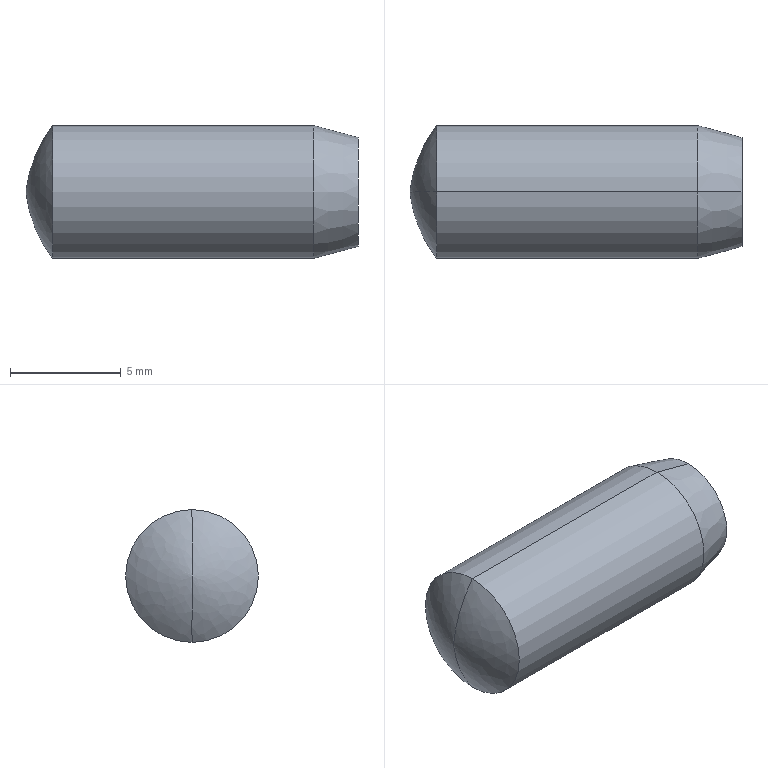Part | STEP file | 0244_010_MSC6-15 | 1 solid | 7 faces | box 15 x 6 x 6 mm | volume 396.61 mm3 | spline 2 | cylinder 2 | cone 2 | plane 1 | commonest cylinder face diameters 6 x2
STEP:
#1=CARTESIAN_POINT('',(0.,0.,0.));
#2=DIRECTION('',(0.,0.,1.));
#3=DIRECTION('',(1.,0.,0.));
#4=AXIS2_PLACEMENT_3D('',#1,#2,#3);
#5=CARTESIAN_POINT('',(-7.5,0.,0.));
#6=VERTEX_POINT('',#5);
#7=CARTESIAN_POINT('',(-6.3,0.,3.));
#8=VERTEX_POINT('',#7);
#9=CARTESIAN_POINT('',(-1.535,0.,-0.646));
#10=DIRECTION('',(0.,1.,0.));
#11=DIRECTION('',(0.,0.,1.));
#12=AXIS2_PLACEMENT_3D('',#9,#10,#11);
#13=CIRCLE('',#12,6.);
#14=CARTESIAN_POINT('',(-7.5,0.,0.));
#15=CARTESIAN_POINT('',(-7.5,0.,0.));
#16=CARTESIAN_POINT('',(-7.5,0.,0.));
#17=CARTESIAN_POINT('',(-7.5,0.,0.));
#18=CARTESIAN_POINT('',(-7.381,0.,-1.098));
#19=CARTESIAN_POINT('',(-7.381,-2.196,-1.098));
#20=CARTESIAN_POINT('',(-7.381,-2.196,1.098));
#21=CARTESIAN_POINT('',(-7.381,0.,1.098));
#22=CARTESIAN_POINT('',(-6.971,0.,-2.123));
#23=CARTESIAN_POINT('',(-6.971,-4.246,-2.123));
#24=CARTESIAN_POINT('',(-6.971,-4.246,2.123));
#25=CARTESIAN_POINT('',(-6.971,0.,2.123));
#26=CARTESIAN_POINT('',(-6.3,0.,-3.));
#27=CARTESIAN_POINT('',(-6.3,-6.,-3.));
#28=CARTESIAN_POINT('',(-6.3,-6.,3.));
#29=CARTESIAN_POINT('',(-6.3,0.,3.));
#30=(BOUNDED_SURFACE()B_SPLINE_SURFACE(3,3,((#14,#15,#16,#17),(#18,#19,#20,#21),(#22,#23,#24,#25),(#26,#27,#28,#29)),.UNSPECIFIED.,.F.,.F.,.F.)B_SPLINE_SURFACE_WITH_KNOTS((4,4),(4,4),(0.,1.),(0.,1.),.PIECEWISE_BEZIER_KNOTS.)GEOMETRIC_REPRESENTATION_ITEM()RATIONAL_B_SPLINE_SURFACE(((1.,0.3333,0.3333,1.),(0.9754,0.3251,0.3251,0.9754),(0.9754,0.3251,0.3251,0.9754),(1.,0.3333,0.3333,1.)))REPRESENTATION_ITEM('')SURFACE());
#31=CARTESIAN_POINT('',(0.,1.));
#32=CARTESIAN_POINT('',(0.01534,1.));
#33=CARTESIAN_POINT('',(0.04597,1.));
#34=CARTESIAN_POINT('',(0.09177,1.));
#35=CARTESIAN_POINT('',(0.1374,1.));
#36=CARTESIAN_POINT('',(0.183,1.));
#37=CARTESIAN_POINT('',(0.2285,1.));
#38=CARTESIAN_POINT('',(0.2739,1.));
#39=CARTESIAN_POINT('',(0.3192,1.));
#40=CARTESIAN_POINT('',(0.3644,1.));
#41=CARTESIAN_POINT('',(0.4096,1.));
#42=CARTESIAN_POINT('',(0.4548,1.));
#43=CARTESIAN_POINT('',(0.5,1.));
#44=CARTESIAN_POINT('',(0.5452,1.));
#45=CARTESIAN_POINT('',(0.5904,1.));
#46=CARTESIAN_POINT('',(0.6356,1.));
#47=CARTESIAN_POINT('',(0.6808,1.));
#48=CARTESIAN_POINT('',(0.7261,1.));
#49=CARTESIAN_POINT('',(0.7715,1.));
#50=CARTESIAN_POINT('',(0.817,1.));
#51=CARTESIAN_POINT('',(0.8626,1.));
#52=CARTESIAN_POINT('',(0.9082,1.));
#53=CARTESIAN_POINT('',(0.954,1.));
#54=CARTESIAN_POINT('',(0.9847,1.));
#55=CARTESIAN_POINT('',(1.,1.));
#56=B_SPLINE_CURVE_WITH_KNOTS('',3,(#31,#32,#33,#34,#35,#36,#37,#38,#39,#40,#41,#42,#43,#44,#45,#46,#47,#48,#49,#50,#51,#52,#53,#54,#55),.UNSPECIFIED.,.F.,.F.,(4,1,1,1,1,1,1,1,1,1,1,1,1,1,1,1,1,1,1,1,1,1,4),(4.82,4.845,4.87,4.895,4.919,4.944,4.969,4.994,5.019,5.043,5.068,5.093,5.118,5.142,5.167,5.192,5.217,5.242,5.266,5.291,5.316,5.341,5.366),.QUASI_UNIFORM_KNOTS.);
#57=(GEOMETRIC_REPRESENTATION_CONTEXT(2)PARAMETRIC_REPRESENTATION_CONTEXT()REPRESENTATION_CONTEXT('',''));
#58=DEFINITIONAL_REPRESENTATION('',(#56),#57);
#59=PCURVE('',#30,#58);
#60=CARTESIAN_POINT('',(-7.5,0.,0.));
#61=CARTESIAN_POINT('',(-7.5,0.,0.));
#62=CARTESIAN_POINT('',(-7.5,0.,0.));
#63=CARTESIAN_POINT('',(-7.5,0.,0.));
#64=CARTESIAN_POINT('',(-7.381,0.,1.098));
#65=CARTESIAN_POINT('',(-7.381,2.196,1.098));
#66=CARTESIAN_POINT('',(-7.381,2.196,-1.098));
#67=CARTESIAN_POINT('',(-7.381,0.,-1.098));
#68=CARTESIAN_POINT('',(-6.971,0.,2.123));
#69=CARTESIAN_POINT('',(-6.971,4.246,2.123));
#70=CARTESIAN_POINT('',(-6.971,4.246,-2.123));
#71=CARTESIAN_POINT('',(-6.971,0.,-2.123));
#72=CARTESIAN_POINT('',(-6.3,0.,3.));
#73=CARTESIAN_POINT('',(-6.3,6.,3.));
#74=CARTESIAN_POINT('',(-6.3,6.,-3.));
#75=CARTESIAN_POINT('',(-6.3,0.,-3.));
#76=(BOUNDED_SURFACE()B_SPLINE_SURFACE(3,3,((#60,#61,#62,#63),(#64,#65,#66,#67),(#68,#69,#70,#71),(#72,#73,#74,#75)),.UNSPECIFIED.,.F.,.F.,.F.)B_SPLINE_SURFACE_WITH_KNOTS((4,4),(4,4),(0.,1.),(0.,1.),.PIECEWISE_BEZIER_KNOTS.)GEOMETRIC_REPRESENTATION_ITEM()RATIONAL_B_SPLINE_SURFACE(((1.,0.3333,0.3333,1.),(0.9754,0.3251,0.3251,0.9754),(0.9754,0.3251,0.3251,0.9754),(1.,0.3333,0.3333,1.)))REPRESENTATION_ITEM('')SURFACE());
#77=CARTESIAN_POINT('',(0.,0.));
#78=CARTESIAN_POINT('',(0.01534,0.));
#79=CARTESIAN_POINT('',(0.04597,0.));
#80=CARTESIAN_POINT('',(0.09177,0.));
#81=CARTESIAN_POINT('',(0.1374,0.));
#82=CARTESIAN_POINT('',(0.183,0.));
#83=CARTESIAN_POINT('',(0.2285,0.));
#84=CARTESIAN_POINT('',(0.2739,0.));
#85=CARTESIAN_POINT('',(0.3192,0.));
#86=CARTESIAN_POINT('',(0.3644,0.));
#87=CARTESIAN_POINT('',(0.4096,0.));
#88=CARTESIAN_POINT('',(0.4548,0.));
#89=CARTESIAN_POINT('',(0.5,0.));
#90=CARTESIAN_POINT('',(0.5452,0.));
#91=CARTESIAN_POINT('',(0.5904,0.));
#92=CARTESIAN_POINT('',(0.6356,0.));
#93=CARTESIAN_POINT('',(0.6808,0.));
#94=CARTESIAN_POINT('',(0.7261,0.));
#95=CARTESIAN_POINT('',(0.7715,0.));
#96=CARTESIAN_POINT('',(0.817,0.));
#97=CARTESIAN_POINT('',(0.8626,0.));
#98=CARTESIAN_POINT('',(0.9082,0.));
#99=CARTESIAN_POINT('',(0.954,0.));
#100=CARTESIAN_POINT('',(0.9847,0.));
#101=CARTESIAN_POINT('',(1.,0.));
#102=B_SPLINE_CURVE_WITH_KNOTS('',3,(#77,#78,#79,#80,#81,#82,#83,#84,#85,#86,#87,#88,#89,#90,#91,#92,#93,#94,#95,#96,#97,#98,#99,#100,#101),.UNSPECIFIED.,.F.,.F.,(4,1,1,1,1,1,1,1,1,1,1,1,1,1,1,1,1,1,1,1,1,1,4),(4.82,4.845,4.87,4.895,4.919,4.944,4.969,4.994,5.019,5.043,5.068,5.093,5.118,5.142,5.167,5.192,5.217,5.242,5.266,5.291,5.316,5.341,5.366),.QUASI_UNIFORM_KNOTS.);
#103=(GEOMETRIC_REPRESENTATION_CONTEXT(2)PARAMETRIC_REPRESENTATION_CONTEXT()REPRESENTATION_CONTEXT('',''));
#104=DEFINITIONAL_REPRESENTATION('',(#102),#103);
#105=PCURVE('',#76,#104);
#106=SURFACE_CURVE('',#13,(#59,#105),.PCURVE_S1.);
#107=EDGE_CURVE('',#6,#8,#106,.T.);
#108=ORIENTED_EDGE('',*,*,#107,.F.);
#109=CARTESIAN_POINT('',(-6.3,0.,-3.));
#110=VERTEX_POINT('',#109);
#111=CARTESIAN_POINT('',(-1.535,0.,0.646));
#112=DIRECTION('',(0.,-1.,0.));
#113=DIRECTION('',(0.,0.,-1.));
#114=AXIS2_PLACEMENT_3D('',#111,#112,#113);
#115=CIRCLE('',#114,6.);
#116=CARTESIAN_POINT('',(0.,0.));
#117=CARTESIAN_POINT('',(0.01534,0.));
#118=CARTESIAN_POINT('',(0.04597,0.));
#119=CARTESIAN_POINT('',(0.09177,0.));
#120=CARTESIAN_POINT('',(0.1374,0.));
#121=CARTESIAN_POINT('',(0.183,0.));
#122=CARTESIAN_POINT('',(0.2285,0.));
#123=CARTESIAN_POINT('',(0.2739,0.));
#124=CARTESIAN_POINT('',(0.3192,0.));
#125=CARTESIAN_POINT('',(0.3644,0.));
#126=CARTESIAN_POINT('',(0.4096,0.));
#127=CARTESIAN_POINT('',(0.4548,0.));
#128=CARTESIAN_POINT('',(0.5,0.));
#129=CARTESIAN_POINT('',(0.5452,0.));
#130=CARTESIAN_POINT('',(0.5904,0.));
#131=CARTESIAN_POINT('',(0.6356,0.));
#132=CARTESIAN_POINT('',(0.6808,0.));
#133=CARTESIAN_POINT('',(0.7261,0.));
#134=CARTESIAN_POINT('',(0.7715,0.));
#135=CARTESIAN_POINT('',(0.817,0.));
#136=CARTESIAN_POINT('',(0.8626,0.));
#137=CARTESIAN_POINT('',(0.9082,0.));
#138=CARTESIAN_POINT('',(0.954,0.));
#139=CARTESIAN_POINT('',(0.9847,0.));
#140=CARTESIAN_POINT('',(1.,0.));
#141=B_SPLINE_CURVE_WITH_KNOTS('',3,(#116,#117,#118,#119,#120,#121,#122,#123,#124,#125,#126,#127,#128,#129,#130,#131,#132,#133,#134,#135,#136,#137,#138,#139,#140),.UNSPECIFIED.,.F.,.F.,(4,1,1,1,1,1,1,1,1,1,1,1,1,1,1,1,1,1,1,1,1,1,4),(4.82,4.845,4.87,4.895,4.919,4.944,4.969,4.994,5.019,5.043,5.068,5.093,5.118,5.142,5.167,5.192,5.217,5.242,5.266,5.291,5.316,5.341,5.366),.QUASI_UNIFORM_KNOTS.);
#142=(GEOMETRIC_REPRESENTATION_CONTEXT(2)PARAMETRIC_REPRESENTATION_CONTEXT()REPRESENTATION_CONTEXT('',''));
#143=DEFINITIONAL_REPRESENTATION('',(#141),#142);
#144=PCURVE('',#30,#143);
#145=CARTESIAN_POINT('',(0.,1.));
#146=CARTESIAN_POINT('',(0.01534,1.));
#147=CARTESIAN_POINT('',(0.04597,1.));
#148=CARTESIAN_POINT('',(0.09177,1.));
#149=CARTESIAN_POINT('',(0.1374,1.));
#150=CARTESIAN_POINT('',(0.183,1.));
#151=CARTESIAN_POINT('',(0.2285,1.));
#152=CARTESIAN_POINT('',(0.2739,1.));
#153=CARTESIAN_POINT('',(0.3192,1.));
#154=CARTESIAN_POINT('',(0.3644,1.));
#155=CARTESIAN_POINT('',(0.4096,1.));
#156=CARTESIAN_POINT('',(0.4548,1.));
#157=CARTESIAN_POINT('',(0.5,1.));
#158=CARTESIAN_POINT('',(0.5452,1.));
#159=CARTESIAN_POINT('',(0.5904,1.));
#160=CARTESIAN_POINT('',(0.6356,1.));
#161=CARTESIAN_POINT('',(0.6808,1.));
#162=CARTESIAN_POINT('',(0.7261,1.));
#163=CARTESIAN_POINT('',(0.7715,1.));
#164=CARTESIAN_POINT('',(0.817,1.));
#165=CARTESIAN_POINT('',(0.8626,1.));
#166=CARTESIAN_POINT('',(0.9082,1.));
#167=CARTESIAN_POINT('',(0.954,1.));
#168=CARTESIAN_POINT('',(0.9847,1.));
#169=CARTESIAN_POINT('',(1.,1.));
#170=B_SPLINE_CURVE_WITH_KNOTS('',3,(#145,#146,#147,#148,#149,#150,#151,#152,#153,#154,#155,#156,#157,#158,#159,#160,#161,#162,#163,#164,#165,#166,#167,#168,#169),.UNSPECIFIED.,.F.,.F.,(4,1,1,1,1,1,1,1,1,1,1,1,1,1,1,1,1,1,1,1,1,1,4),(4.82,4.845,4.87,4.895,4.919,4.944,4.969,4.994,5.019,5.043,5.068,5.093,5.118,5.142,5.167,5.192,5.217,5.242,5.266,5.291,5.316,5.341,5.366),.QUASI_UNIFORM_KNOTS.);
#171=(GEOMETRIC_REPRESENTATION_CONTEXT(2)PARAMETRIC_REPRESENTATION_CONTEXT()REPRESENTATION_CONTEXT('',''));
#172=DEFINITIONAL_REPRESENTATION('',(#170),#171);
#173=PCURVE('',#76,#172);
#174=SURFACE_CURVE('',#115,(#144,#173),.PCURVE_S1.);
#175=EDGE_CURVE('',#6,#110,#174,.T.);
#176=ORIENTED_EDGE('',*,*,#175,.T.);
#177=CARTESIAN_POINT('',(-6.3,0.,0.));
#178=DIRECTION('',(1.,0.,0.));
#179=DIRECTION('',(0.,0.,-1.));
#180=AXIS2_PLACEMENT_3D('',#177,#178,#179);
#181=CIRCLE('',#180,3.);
#182=CARTESIAN_POINT('',(1.,1.));
#183=CARTESIAN_POINT('',(1.,0.9763));
#184=CARTESIAN_POINT('',(1.,0.9319));
#185=CARTESIAN_POINT('',(1.,0.8733));
#186=CARTESIAN_POINT('',(1.,0.8206));
#187=CARTESIAN_POINT('',(1.,0.7724));
#188=CARTESIAN_POINT('',(1.,0.7279));
#189=CARTESIAN_POINT('',(1.,0.6861));
#190=CARTESIAN_POINT('',(1.,0.6465));
#191=CARTESIAN_POINT('',(1.,0.6086));
#192=CARTESIAN_POINT('',(1.,0.5718));
#193=CARTESIAN_POINT('',(1.,0.5357));
#194=CARTESIAN_POINT('',(1.,0.5));
#195=CARTESIAN_POINT('',(1.,0.4643));
#196=CARTESIAN_POINT('',(1.,0.4282));
#197=CARTESIAN_POINT('',(1.,0.3914));
#198=CARTESIAN_POINT('',(1.,0.3535));
#199=CARTESIAN_POINT('',(1.,0.3139));
#200=CARTESIAN_POINT('',(1.,0.2721));
#201=CARTESIAN_POINT('',(1.,0.2276));
#202=CARTESIAN_POINT('',(1.,0.1794));
#203=CARTESIAN_POINT('',(1.,0.1267));
#204=CARTESIAN_POINT('',(1.,0.06805));
#205=CARTESIAN_POINT('',(1.,0.02375));
#206=CARTESIAN_POINT('',(1.,0.));
#207=B_SPLINE_CURVE_WITH_KNOTS('',3,(#182,#183,#184,#185,#186,#187,#188,#189,#190,#191,#192,#193,#194,#195,#196,#197,#198,#199,#200,#201,#202,#203,#204,#205,#206),.UNSPECIFIED.,.F.,.F.,(4,1,1,1,1,1,1,1,1,1,1,1,1,1,1,1,1,1,1,1,1,1,4),(3.142,3.284,3.427,3.57,3.713,3.856,3.998,4.141,4.284,4.427,4.57,4.712,4.855,4.998,5.141,5.284,5.426,5.569,5.712,5.855,5.998,6.14,6.283),.QUASI_UNIFORM_KNOTS.);
#208=(GEOMETRIC_REPRESENTATION_CONTEXT(2)PARAMETRIC_REPRESENTATION_CONTEXT()REPRESENTATION_CONTEXT('',''));
#209=DEFINITIONAL_REPRESENTATION('',(#207),#208);
#210=PCURVE('',#30,#209);
#211=CARTESIAN_POINT('',(-0.4,0.,0.));
#212=DIRECTION('',(1.,0.,0.));
#213=DIRECTION('',(0.,0.,-1.));
#214=AXIS2_PLACEMENT_3D('',#211,#212,#213);
#215=CYLINDRICAL_SURFACE('',#214,3.);
#216=CARTESIAN_POINT('',(0.,-5.9));
#217=DIRECTION('',(1.,0.));
#218=VECTOR('',#217,1.);
#219=LINE('',#216,#218);
#220=(GEOMETRIC_REPRESENTATION_CONTEXT(2)PARAMETRIC_REPRESENTATION_CONTEXT()REPRESENTATION_CONTEXT('',''));
#221=DEFINITIONAL_REPRESENTATION('',(#219),#220);
#222=PCURVE('',#215,#221);
#223=SURFACE_CURVE('',#181,(#210,#222),.PCURVE_S1.);
#224=EDGE_CURVE('',#8,#110,#223,.T.);
#225=ORIENTED_EDGE('',*,*,#224,.F.);
#226=EDGE_LOOP('',(#108,#176,#225));
#227=FACE_BOUND('',#226,.T.);
#228=ADVANCED_FACE('',(#227),#30,.T.);
#229=CARTESIAN_POINT('',(-6.3,0.,0.));
#230=DIRECTION('',(1.,0.,0.));
#231=DIRECTION('',(0.,0.,-1.));
#232=AXIS2_PLACEMENT_3D('',#229,#230,#231);
#233=CIRCLE('',#232,3.);
#234=CARTESIAN_POINT('',(-0.4,0.,0.));
#235=DIRECTION('',(1.,0.,0.));
#236=DIRECTION('',(0.,0.,-1.));
#237=AXIS2_PLACEMENT_3D('',#234,#235,#236);
#238=CYLINDRICAL_SURFACE('',#237,3.);
#239=CARTESIAN_POINT('',(0.,-5.9));
#240=DIRECTION('',(1.,0.));
#241=VECTOR('',#240,1.);
#242=LINE('',#239,#241);
#243=(GEOMETRIC_REPRESENTATION_CONTEXT(2)PARAMETRIC_REPRESENTATION_CONTEXT()REPRESENTATION_CONTEXT('',''));
#244=DEFINITIONAL_REPRESENTATION('',(#242),#243);
#245=PCURVE('',#238,#244);
#246=CARTESIAN_POINT('',(1.,1.));
#247=CARTESIAN_POINT('',(1.,0.9763));
#248=CARTESIAN_POINT('',(1.,0.9319));
#249=CARTESIAN_POINT('',(1.,0.8733));
#250=CARTESIAN_POINT('',(1.,0.8206));
#251=CARTESIAN_POINT('',(1.,0.7724));
#252=CARTESIAN_POINT('',(1.,0.7279));
#253=CARTESIAN_POINT('',(1.,0.6861));
#254=CARTESIAN_POINT('',(1.,0.6465));
#255=CARTESIAN_POINT('',(1.,0.6086));
#256=CARTESIAN_POINT('',(1.,0.5718));
#257=CARTESIAN_POINT('',(1.,0.5357));
#258=CARTESIAN_POINT('',(1.,0.5));
#259=CARTESIAN_POINT('',(1.,0.4643));
#260=CARTESIAN_POINT('',(1.,0.4282));
#261=CARTESIAN_POINT('',(1.,0.3914));
#262=CARTESIAN_POINT('',(1.,0.3535));
#263=CARTESIAN_POINT('',(1.,0.3139));
#264=CARTESIAN_POINT('',(1.,0.2721));
#265=CARTESIAN_POINT('',(1.,0.2276));
#266=CARTESIAN_POINT('',(1.,0.1794));
#267=CARTESIAN_POINT('',(1.,0.1267));
#268=CARTESIAN_POINT('',(1.,0.06805));
#269=CARTESIAN_POINT('',(1.,0.02375));
#270=CARTESIAN_POINT('',(1.,0.));
#271=B_SPLINE_CURVE_WITH_KNOTS('',3,(#246,#247,#248,#249,#250,#251,#252,#253,#254,#255,#256,#257,#258,#259,#260,#261,#262,#263,#264,#265,#266,#267,#268,#269,#270),.UNSPECIFIED.,.F.,.F.,(4,1,1,1,1,1,1,1,1,1,1,1,1,1,1,1,1,1,1,1,1,1,4),(0.,0.1428,0.2856,0.4284,0.5712,0.714,0.8568,0.9996,1.142,1.285,1.428,1.571,1.714,1.856,1.999,2.142,2.285,2.428,2.57,2.713,2.856,2.999,3.142),.QUASI_UNIFORM_KNOTS.);
#272=(GEOMETRIC_REPRESENTATION_CONTEXT(2)PARAMETRIC_REPRESENTATION_CONTEXT()REPRESENTATION_CONTEXT('',''));
#273=DEFINITIONAL_REPRESENTATION('',(#271),#272);
#274=PCURVE('',#76,#273);
#275=SURFACE_CURVE('',#233,(#245,#274),.PCURVE_S1.);
#276=EDGE_CURVE('',#110,#8,#275,.T.);
#277=ORIENTED_EDGE('',*,*,#276,.T.);
#278=CARTESIAN_POINT('',(5.5,0.,3.));
#279=VERTEX_POINT('',#278);
#280=CARTESIAN_POINT('',(-0.4,0.,3.));
#281=DIRECTION('',(1.,0.,0.));
#282=VECTOR('',#281,1.);
#283=LINE('',#280,#282);
#284=CARTESIAN_POINT('',(3.142,0.));
#285=DIRECTION('',(0.,1.));
#286=VECTOR('',#285,1.);
#287=LINE('',#284,#286);
#288=(GEOMETRIC_REPRESENTATION_CONTEXT(2)PARAMETRIC_REPRESENTATION_CONTEXT()REPRESENTATION_CONTEXT('',''));
#289=DEFINITIONAL_REPRESENTATION('',(#287),#288);
#290=PCURVE('',#238,#289);
#291=CARTESIAN_POINT('',(3.142,0.));
#292=DIRECTION('',(0.,1.));
#293=VECTOR('',#292,1.);
#294=LINE('',#291,#293);
#295=(GEOMETRIC_REPRESENTATION_CONTEXT(2)PARAMETRIC_REPRESENTATION_CONTEXT()REPRESENTATION_CONTEXT('',''));
#296=DEFINITIONAL_REPRESENTATION('',(#294),#295);
#297=PCURVE('',#215,#296);
#298=SURFACE_CURVE('',#283,(#290,#297),.PCURVE_S1.);
#299=EDGE_CURVE('',#8,#279,#298,.T.);
#300=ORIENTED_EDGE('',*,*,#299,.T.);
#301=CARTESIAN_POINT('',(5.5,0.,-3.));
#302=VERTEX_POINT('',#301);
#303=CARTESIAN_POINT('',(5.5,0.,0.));
#304=DIRECTION('',(-1.,0.,0.));
#305=DIRECTION('',(0.,0.,-1.));
#306=AXIS2_PLACEMENT_3D('',#303,#304,#305);
#307=CIRCLE('',#306,3.);
#308=CARTESIAN_POINT('',(6.283,5.9));
#309=DIRECTION('',(-1.,0.));
#310=VECTOR('',#309,1.);
#311=LINE('',#308,#310);
#312=(GEOMETRIC_REPRESENTATION_CONTEXT(2)PARAMETRIC_REPRESENTATION_CONTEXT()REPRESENTATION_CONTEXT('',''));
#313=DEFINITIONAL_REPRESENTATION('',(#311),#312);
#314=PCURVE('',#238,#313);
#315=CARTESIAN_POINT('',(5.5,0.,0.));
#316=DIRECTION('',(-1.,0.,0.));
#317=DIRECTION('',(0.,0.,1.));
#318=AXIS2_PLACEMENT_3D('',#315,#316,#317);
#319=CONICAL_SURFACE('',#318,3.,0.2618);
#320=CARTESIAN_POINT('',(-3.142,0.));
#321=DIRECTION('',(1.,0.));
#322=VECTOR('',#321,1.);
#323=LINE('',#320,#322);
#324=(GEOMETRIC_REPRESENTATION_CONTEXT(2)PARAMETRIC_REPRESENTATION_CONTEXT()REPRESENTATION_CONTEXT('',''));
#325=DEFINITIONAL_REPRESENTATION('',(#323),#324);
#326=PCURVE('',#319,#325);
#327=SURFACE_CURVE('',#307,(#314,#326),.PCURVE_S1.);
#328=EDGE_CURVE('',#279,#302,#327,.T.);
#329=ORIENTED_EDGE('',*,*,#328,.T.);
#330=CARTESIAN_POINT('',(-0.4,0.,-3.));
#331=DIRECTION('',(1.,0.,0.));
#332=VECTOR('',#331,1.);
#333=LINE('',#330,#332);
#334=CARTESIAN_POINT('',(0.,0.));
#335=DIRECTION('',(0.,1.));
#336=VECTOR('',#335,1.);
#337=LINE('',#334,#336);
#338=(GEOMETRIC_REPRESENTATION_CONTEXT(2)PARAMETRIC_REPRESENTATION_CONTEXT()REPRESENTATION_CONTEXT('',''));
#339=DEFINITIONAL_REPRESENTATION('',(#337),#338);
#340=PCURVE('',#238,#339);
#341=CARTESIAN_POINT('',(6.283,0.));
#342=DIRECTION('',(0.,1.));
#343=VECTOR('',#342,1.);
#344=LINE('',#341,#343);
#345=(GEOMETRIC_REPRESENTATION_CONTEXT(2)PARAMETRIC_REPRESENTATION_CONTEXT()REPRESENTATION_CONTEXT('',''));
#346=DEFINITIONAL_REPRESENTATION('',(#344),#345);
#347=PCURVE('',#215,#346);
#348=SURFACE_CURVE('',#333,(#340,#347),.PCURVE_S1.);
#349=EDGE_CURVE('',#110,#302,#348,.T.);
#350=ORIENTED_EDGE('',*,*,#349,.F.);
#351=EDGE_LOOP('',(#277,#300,#329,#350));
#352=FACE_BOUND('',#351,.T.);
#353=ADVANCED_FACE('',(#352),#238,.T.);
#354=CARTESIAN_POINT('',(7.5,0.,2.464));
#355=VERTEX_POINT('',#354);
#356=CARTESIAN_POINT('',(7.5,0.,-2.464));
#357=VERTEX_POINT('',#356);
#358=CARTESIAN_POINT('',(7.5,0.,0.));
#359=DIRECTION('',(-1.,0.,0.));
#360=DIRECTION('',(0.,0.,1.));
#361=AXIS2_PLACEMENT_3D('',#358,#359,#360);
#362=CIRCLE('',#361,2.464);
#363=CARTESIAN_POINT('',(0.,-2.));
#364=DIRECTION('',(1.,0.));
#365=VECTOR('',#364,1.);
#366=LINE('',#363,#365);
#367=(GEOMETRIC_REPRESENTATION_CONTEXT(2)PARAMETRIC_REPRESENTATION_CONTEXT()REPRESENTATION_CONTEXT('',''));
#368=DEFINITIONAL_REPRESENTATION('',(#366),#367);
#369=PCURVE('',#319,#368);
#370=CARTESIAN_POINT('',(7.5,1.232,0.));
#371=DIRECTION('',(1.,0.,0.));
#372=DIRECTION('',(0.,0.,-1.));
#373=AXIS2_PLACEMENT_3D('',#370,#371,#372);
#374=PLANE('',#373);
#375=CARTESIAN_POINT('',(-2.464,-1.232));
#376=CARTESIAN_POINT('',(-2.464,3.036));
#377=CARTESIAN_POINT('',(1.232,0.9019));
#378=CARTESIAN_POINT('',(4.928,-1.232));
#379=CARTESIAN_POINT('',(1.232,-3.366));
#380=CARTESIAN_POINT('',(-2.464,-5.5));
#381=CARTESIAN_POINT('',(-2.464,-1.232));
#382=(BOUNDED_CURVE()B_SPLINE_CURVE(2,(#375,#376,#377,#378,#379,#380,#381),.UNSPECIFIED.,.T.,.F.)B_SPLINE_CURVE_WITH_KNOTS((1,2,2,2,2,1),(-2.094,0.,2.094,4.189,6.283,8.378),.UNSPECIFIED.)CURVE()GEOMETRIC_REPRESENTATION_ITEM()RATIONAL_B_SPLINE_CURVE((1.,0.5,1.,0.5,1.,0.5,1.))REPRESENTATION_ITEM(''));
#383=(GEOMETRIC_REPRESENTATION_CONTEXT(2)PARAMETRIC_REPRESENTATION_CONTEXT()REPRESENTATION_CONTEXT('',''));
#384=DEFINITIONAL_REPRESENTATION('',(#382),#383);
#385=PCURVE('',#374,#384);
#386=SURFACE_CURVE('',#362,(#369,#385),.PCURVE_S1.);
#387=EDGE_CURVE('',#355,#357,#386,.T.);
#388=ORIENTED_EDGE('',*,*,#387,.T.);
#389=CARTESIAN_POINT('',(5.5,0.,-3.));
#390=DIRECTION('',(-0.9659,0.,-0.2588));
#391=VECTOR('',#390,1.);
#392=LINE('',#389,#391);
#393=CARTESIAN_POINT('',(3.142,0.));
#394=DIRECTION('',(0.,1.));
#395=VECTOR('',#394,1.);
#396=LINE('',#393,#395);
#397=(GEOMETRIC_REPRESENTATION_CONTEXT(2)PARAMETRIC_REPRESENTATION_CONTEXT()REPRESENTATION_CONTEXT('',''));
#398=DEFINITIONAL_REPRESENTATION('',(#396),#397);
#399=PCURVE('',#319,#398);
#400=CARTESIAN_POINT('',(5.5,0.,0.));
#401=DIRECTION('',(-1.,0.,0.));
#402=DIRECTION('',(0.,0.,1.));
#403=AXIS2_PLACEMENT_3D('',#400,#401,#402);
#404=CONICAL_SURFACE('',#403,3.,0.2618);
#405=CARTESIAN_POINT('',(3.142,0.));
#406=DIRECTION('',(0.,1.));
#407=VECTOR('',#406,1.);
#408=LINE('',#405,#407);
#409=(GEOMETRIC_REPRESENTATION_CONTEXT(2)PARAMETRIC_REPRESENTATION_CONTEXT()REPRESENTATION_CONTEXT('',''));
#410=DEFINITIONAL_REPRESENTATION('',(#408),#409);
#411=PCURVE('',#404,#410);
#412=SURFACE_CURVE('',#392,(#399,#411),.PCURVE_S1.);
#413=EDGE_CURVE('',#357,#302,#412,.T.);
#414=ORIENTED_EDGE('',*,*,#413,.T.);
#415=ORIENTED_EDGE('',*,*,#328,.F.);
#416=CARTESIAN_POINT('',(5.5,0.,3.));
#417=DIRECTION('',(-0.9659,0.,0.2588));
#418=VECTOR('',#417,1.);
#419=LINE('',#416,#418);
#420=CARTESIAN_POINT('',(0.,0.));
#421=DIRECTION('',(0.,1.));
#422=VECTOR('',#421,1.);
#423=LINE('',#420,#422);
#424=(GEOMETRIC_REPRESENTATION_CONTEXT(2)PARAMETRIC_REPRESENTATION_CONTEXT()REPRESENTATION_CONTEXT('',''));
#425=DEFINITIONAL_REPRESENTATION('',(#423),#424);
#426=PCURVE('',#319,#425);
#427=CARTESIAN_POINT('',(6.283,0.));
#428=DIRECTION('',(0.,1.));
#429=VECTOR('',#428,1.);
#430=LINE('',#427,#429);
#431=(GEOMETRIC_REPRESENTATION_CONTEXT(2)PARAMETRIC_REPRESENTATION_CONTEXT()REPRESENTATION_CONTEXT('',''));
#432=DEFINITIONAL_REPRESENTATION('',(#430),#431);
#433=PCURVE('',#404,#432);
#434=SURFACE_CURVE('',#419,(#426,#433),.PCURVE_S1.);
#435=EDGE_CURVE('',#355,#279,#434,.T.);
#436=ORIENTED_EDGE('',*,*,#435,.F.);
#437=EDGE_LOOP('',(#388,#414,#415,#436));
#438=FACE_BOUND('',#437,.T.);
#439=ADVANCED_FACE('',(#438),#319,.T.);
#440=ORIENTED_EDGE('',*,*,#299,.F.);
#441=ORIENTED_EDGE('',*,*,#224,.T.);
#442=ORIENTED_EDGE('',*,*,#349,.T.);
#443=CARTESIAN_POINT('',(5.5,0.,0.));
#444=DIRECTION('',(-1.,0.,0.));
#445=DIRECTION('',(0.,0.,-1.));
#446=AXIS2_PLACEMENT_3D('',#443,#444,#445);
#447=CIRCLE('',#446,3.);
#448=CARTESIAN_POINT('',(6.283,5.9));
#449=DIRECTION('',(-1.,0.));
#450=VECTOR('',#449,1.);
#451=LINE('',#448,#450);
#452=(GEOMETRIC_REPRESENTATION_CONTEXT(2)PARAMETRIC_REPRESENTATION_CONTEXT()REPRESENTATION_CONTEXT('',''));
#453=DEFINITIONAL_REPRESENTATION('',(#451),#452);
#454=PCURVE('',#215,#453);
#455=CARTESIAN_POINT('',(3.142,0.));
#456=DIRECTION('',(1.,0.));
#457=VECTOR('',#456,1.);
#458=LINE('',#455,#457);
#459=(GEOMETRIC_REPRESENTATION_CONTEXT(2)PARAMETRIC_REPRESENTATION_CONTEXT()REPRESENTATION_CONTEXT('',''));
#460=DEFINITIONAL_REPRESENTATION('',(#458),#459);
#461=PCURVE('',#404,#460);
#462=SURFACE_CURVE('',#447,(#454,#461),.PCURVE_S1.);
#463=EDGE_CURVE('',#302,#279,#462,.T.);
#464=ORIENTED_EDGE('',*,*,#463,.T.);
#465=EDGE_LOOP('',(#440,#441,#442,#464));
#466=FACE_BOUND('',#465,.T.);
#467=ADVANCED_FACE('',(#466),#215,.T.);
#468=ORIENTED_EDGE('',*,*,#175,.F.);
#469=ORIENTED_EDGE('',*,*,#107,.T.);
#470=ORIENTED_EDGE('',*,*,#276,.F.);
#471=EDGE_LOOP('',(#468,#469,#470));
#472=FACE_BOUND('',#471,.T.);
#473=ADVANCED_FACE('',(#472),#76,.T.);
#474=ORIENTED_EDGE('',*,*,#413,.F.);
#475=CARTESIAN_POINT('',(7.5,0.,0.));
#476=DIRECTION('',(-1.,0.,0.));
#477=DIRECTION('',(0.,0.,1.));
#478=AXIS2_PLACEMENT_3D('',#475,#476,#477);
#479=CIRCLE('',#478,2.464);
#480=CARTESIAN_POINT('',(0.,-2.));
#481=DIRECTION('',(1.,0.));
#482=VECTOR('',#481,1.);
#483=LINE('',#480,#482);
#484=(GEOMETRIC_REPRESENTATION_CONTEXT(2)PARAMETRIC_REPRESENTATION_CONTEXT()REPRESENTATION_CONTEXT('',''));
#485=DEFINITIONAL_REPRESENTATION('',(#483),#484);
#486=PCURVE('',#404,#485);
#487=CARTESIAN_POINT('',(-2.464,-1.232));
#488=CARTESIAN_POINT('',(-2.464,3.036));
#489=CARTESIAN_POINT('',(1.232,0.9019));
#490=CARTESIAN_POINT('',(4.928,-1.232));
#491=CARTESIAN_POINT('',(1.232,-3.366));
#492=CARTESIAN_POINT('',(-2.464,-5.5));
#493=CARTESIAN_POINT('',(-2.464,-1.232));
#494=(BOUNDED_CURVE()B_SPLINE_CURVE(2,(#487,#488,#489,#490,#491,#492,#493),.UNSPECIFIED.,.T.,.F.)B_SPLINE_CURVE_WITH_KNOTS((1,2,2,2,2,1),(-2.094,0.,2.094,4.189,6.283,8.378),.UNSPECIFIED.)CURVE()GEOMETRIC_REPRESENTATION_ITEM()RATIONAL_B_SPLINE_CURVE((1.,0.5,1.,0.5,1.,0.5,1.))REPRESENTATION_ITEM(''));
#495=(GEOMETRIC_REPRESENTATION_CONTEXT(2)PARAMETRIC_REPRESENTATION_CONTEXT()REPRESENTATION_CONTEXT('',''));
#496=DEFINITIONAL_REPRESENTATION('',(#494),#495);
#497=PCURVE('',#374,#496);
#498=SURFACE_CURVE('',#479,(#486,#497),.PCURVE_S1.);
#499=EDGE_CURVE('',#357,#355,#498,.T.);
#500=ORIENTED_EDGE('',*,*,#499,.T.);
#501=ORIENTED_EDGE('',*,*,#435,.T.);
#502=ORIENTED_EDGE('',*,*,#463,.F.);
#503=EDGE_LOOP('',(#474,#500,#501,#502));
#504=FACE_BOUND('',#503,.T.);
#505=ADVANCED_FACE('',(#504),#404,.T.);
#506=ORIENTED_EDGE('',*,*,#387,.F.);
#507=ORIENTED_EDGE('',*,*,#499,.F.);
#508=EDGE_LOOP('',(#506,#507));
#509=FACE_BOUND('',#508,.T.);
#510=ADVANCED_FACE('',(#509),#374,.T.);
#511=CLOSED_SHELL('',(#228,#353,#439,#467,#473,#505,#510));
#512=MANIFOLD_SOLID_BREP('',#511);
#513=(LENGTH_UNIT()NAMED_UNIT(*)SI_UNIT(.MILLI.,.METRE.));
#514=UNCERTAINTY_MEASURE_WITH_UNIT(LENGTH_MEASURE(0.0000001),#513,'','');
#515=(NAMED_UNIT(*)PLANE_ANGLE_UNIT()SI_UNIT($,.RADIAN.));
#516=(NAMED_UNIT(*)SI_UNIT($,.STERADIAN.)SOLID_ANGLE_UNIT());
#517=(GEOMETRIC_REPRESENTATION_CONTEXT(3)GLOBAL_UNCERTAINTY_ASSIGNED_CONTEXT((#514))GLOBAL_UNIT_ASSIGNED_CONTEXT((#513,#515,#516))REPRESENTATION_CONTEXT('',''));
#518=ADVANCED_BREP_SHAPE_REPRESENTATION('',(#4,#512),#517);